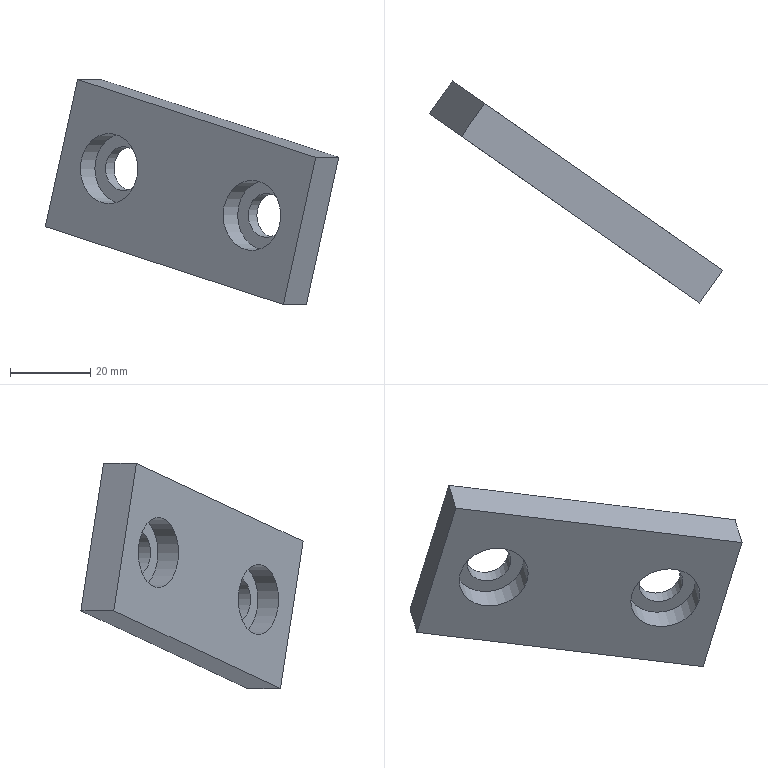Part | NX | features solid 2 | 1 solid | 12 faces | box 73.135 x 55.385 x 56.117 mm | volume 24766 mm3 | plane 8 | cylinder 4 | commonest cylinder face diameters 11 x2 17.5 x2
STEP:
#1=CARTESIAN_POINT('',(-660.026,230.842,18.06));
#2=VERTEX_POINT('',#1);
#3=CARTESIAN_POINT('',(-651.969,225.201,54.765));
#4=VERTEX_POINT('',#3);
#5=CARTESIAN_POINT('',(-681.651,245.984,-80.464));
#6=DIRECTION('',(0.212,-0.1485,0.9659));
#7=VECTOR('',#6,1000.);
#8=LINE('',#5,#7);
#9=EDGE_CURVE('',#2,#4,#8,.T.);
#10=ORIENTED_EDGE('',*,*,#9,.T.);
#11=CARTESIAN_POINT('',(-657.705,217.009,54.765));
#12=VERTEX_POINT('',#11);
#13=CARTESIAN_POINT('',(-396.728,589.724,54.765));
#14=DIRECTION('',(0.5736,0.8192,0.));
#15=VECTOR('',#14,1000.);
#16=LINE('',#13,#15);
#17=EDGE_CURVE('',#12,#4,#16,.T.);
#18=ORIENTED_EDGE('',*,*,#17,.F.);
#19=CARTESIAN_POINT('',(-665.761,222.651,18.06));
#20=VERTEX_POINT('',#19);
#21=CARTESIAN_POINT('',(-687.387,237.793,-80.464));
#22=DIRECTION('',(0.212,-0.1485,0.9659));
#23=VECTOR('',#22,1000.);
#24=LINE('',#21,#23);
#25=EDGE_CURVE('',#20,#12,#24,.T.);
#26=ORIENTED_EDGE('',*,*,#25,.F.);
#27=CARTESIAN_POINT('',(-404.784,595.365,18.06));
#28=DIRECTION('',(0.5736,0.8192,0.));
#29=VECTOR('',#28,1000.);
#30=LINE('',#27,#29);
#31=EDGE_CURVE('',#20,#2,#30,.T.);
#32=ORIENTED_EDGE('',*,*,#31,.T.);
#33=EDGE_LOOP('',(#10,#18,#26,#32));
#34=FACE_BOUND('',#33,.T.);
#35=CARTESIAN_POINT('',(-690.254,233.697,-80.464));
#36=DIRECTION('',(0.7912,-0.554,-0.2588));
#37=DIRECTION('',(-0.5736,-0.8192,0.));
#38=AXIS2_PLACEMENT_3D('',#35,#36,#37);
#39=PLANE('',#38);
#40=ADVANCED_FACE('',(#34),#39,.T.);
#41=CARTESIAN_POINT('',(-719.369,272.394,37.472));
#42=VERTEX_POINT('',#41);
#43=CARTESIAN_POINT('',(-760.909,301.481,51.06));
#44=DIRECTION('',(0.7912,-0.554,-0.2588));
#45=VECTOR('',#44,1000.);
#46=LINE('',#43,#45);
#47=EDGE_CURVE('',#42,#2,#46,.T.);
#48=ORIENTED_EDGE('',*,*,#47,.T.);
#49=ORIENTED_EDGE('',*,*,#31,.F.);
#50=CARTESIAN_POINT('',(-725.104,264.203,37.472));
#51=VERTEX_POINT('',#50);
#52=CARTESIAN_POINT('',(-766.644,293.29,51.06));
#53=DIRECTION('',(0.7912,-0.554,-0.2588));
#54=VECTOR('',#53,1000.);
#55=LINE('',#52,#54);
#56=EDGE_CURVE('',#51,#20,#55,.T.);
#57=ORIENTED_EDGE('',*,*,#56,.F.);
#58=CARTESIAN_POINT('',(-727.972,260.107,37.472));
#59=DIRECTION('',(0.5736,0.8192,0.));
#60=VECTOR('',#59,1000.);
#61=LINE('',#58,#60);
#62=EDGE_CURVE('',#51,#42,#61,.T.);
#63=ORIENTED_EDGE('',*,*,#62,.T.);
#64=EDGE_LOOP('',(#48,#49,#57,#63));
#65=FACE_BOUND('',#64,.T.);
#66=CARTESIAN_POINT('',(-505.667,666.004,51.06));
#67=DIRECTION('',(-0.212,0.1485,-0.9659));
#68=DIRECTION('',(-0.1706,0.9676,0.1862));
#69=AXIS2_PLACEMENT_3D('',#66,#67,#68);
#70=PLANE('',#69);
#71=ADVANCED_FACE('',(#65),#70,.T.);
#72=CARTESIAN_POINT('',(-711.312,266.753,74.177));
#73=VERTEX_POINT('',#72);
#74=CARTESIAN_POINT('',(-731.61,280.966,-18.302));
#75=DIRECTION('',(0.212,-0.1485,0.9659));
#76=VECTOR('',#75,1000.);
#77=LINE('',#74,#76);
#78=EDGE_CURVE('',#42,#73,#77,.T.);
#79=ORIENTED_EDGE('',*,*,#78,.F.);
#80=ORIENTED_EDGE('',*,*,#62,.F.);
#81=CARTESIAN_POINT('',(-717.048,258.562,74.177));
#82=VERTEX_POINT('',#81);
#83=CARTESIAN_POINT('',(-737.346,272.775,-18.302));
#84=DIRECTION('',(0.212,-0.1485,0.9659));
#85=VECTOR('',#84,1000.);
#86=LINE('',#83,#85);
#87=EDGE_CURVE('',#51,#82,#86,.T.);
#88=ORIENTED_EDGE('',*,*,#87,.T.);
#89=CARTESIAN_POINT('',(-719.916,254.466,74.177));
#90=DIRECTION('',(0.5736,0.8192,0.));
#91=VECTOR('',#90,1000.);
#92=LINE('',#89,#91);
#93=EDGE_CURVE('',#82,#73,#92,.T.);
#94=ORIENTED_EDGE('',*,*,#93,.T.);
#95=EDGE_LOOP('',(#79,#80,#88,#94));
#96=FACE_BOUND('',#95,.T.);
#97=CARTESIAN_POINT('',(-749.597,275.249,-61.053));
#98=DIRECTION('',(0.7912,-0.554,-0.2588));
#99=DIRECTION('',(-0.5736,-0.8192,0.));
#100=AXIS2_PLACEMENT_3D('',#97,#98,#99);
#101=PLANE('',#100);
#102=ADVANCED_FACE('',(#96),#101,.F.);
#103=CARTESIAN_POINT('',(-752.852,295.84,87.765));
#104=DIRECTION('',(0.7912,-0.554,-0.2588));
#105=VECTOR('',#104,1000.);
#106=LINE('',#103,#105);
#107=EDGE_CURVE('',#73,#4,#106,.T.);
#108=ORIENTED_EDGE('',*,*,#107,.F.);
#109=ORIENTED_EDGE('',*,*,#93,.F.);
#110=CARTESIAN_POINT('',(-758.588,287.648,87.765));
#111=DIRECTION('',(0.7912,-0.554,-0.2588));
#112=VECTOR('',#111,1000.);
#113=LINE('',#110,#112);
#114=EDGE_CURVE('',#82,#12,#113,.T.);
#115=ORIENTED_EDGE('',*,*,#114,.T.);
#116=ORIENTED_EDGE('',*,*,#17,.T.);
#117=EDGE_LOOP('',(#108,#109,#115,#116));
#118=FACE_BOUND('',#117,.T.);
#119=CARTESIAN_POINT('',(-497.611,660.363,87.765));
#120=DIRECTION('',(-0.212,0.1485,-0.9659));
#121=DIRECTION('',(-0.1706,0.9676,0.1862));
#122=AXIS2_PLACEMENT_3D('',#119,#120,#121);
#123=PLANE('',#122);
#124=ADVANCED_FACE('',(#118),#123,.F.);
#125=CARTESIAN_POINT('',(-680.769,233.159,40.295));
#126=VERTEX_POINT('',#125);
#127=CARTESIAN_POINT('',(-673.602,228.14,40.295));
#128=DIRECTION('',(0.5736,0.8192,0.));
#129=DIRECTION('',(-0.8192,0.5736,0.));
#130=AXIS2_PLACEMENT_3D('',#127,#128,#129);
#131=CIRCLE('',#130,8.75);
#132=EDGE_CURVE('',#126,#126,#131,.T.);
#133=ORIENTED_EDGE('',*,*,#132,.T.);
#134=EDGE_LOOP('',(#133));
#135=FACE_BOUND('',#134,.T.);
#136=CARTESIAN_POINT('',(-716.375,258.091,51.942));
#137=VERTEX_POINT('',#136);
#138=CARTESIAN_POINT('',(-709.207,253.072,51.942));
#139=DIRECTION('',(0.5736,0.8192,0.));
#140=DIRECTION('',(-0.8192,0.5736,0.));
#141=AXIS2_PLACEMENT_3D('',#138,#139,#140);
#142=CIRCLE('',#141,8.75);
#143=EDGE_CURVE('',#137,#137,#142,.T.);
#144=ORIENTED_EDGE('',*,*,#143,.T.);
#145=EDGE_LOOP('',(#144));
#146=FACE_BOUND('',#145,.T.);
#147=ORIENTED_EDGE('',*,*,#25,.T.);
#148=ORIENTED_EDGE('',*,*,#114,.F.);
#149=ORIENTED_EDGE('',*,*,#87,.F.);
#150=ORIENTED_EDGE('',*,*,#56,.T.);
#151=EDGE_LOOP('',(#147,#148,#149,#150));
#152=FACE_BOUND('',#151,.T.);
#153=CARTESIAN_POINT('',(-739.324,274.16,-17.655));
#154=DIRECTION('',(-0.5736,-0.8192,0.));
#155=DIRECTION('',(-0.8192,0.5736,0.));
#156=AXIS2_PLACEMENT_3D('',#153,#154,#155);
#157=PLANE('',#156);
#158=ADVANCED_FACE('',(#135,#146,#152),#157,.T.);
#159=CARTESIAN_POINT('',(-663.361,233.177,40.295));
#160=VERTEX_POINT('',#159);
#161=CARTESIAN_POINT('',(-667.866,236.332,40.295));
#162=DIRECTION('',(-0.5736,-0.8192,0.));
#163=DIRECTION('',(0.8192,-0.5736,0.));
#164=AXIS2_PLACEMENT_3D('',#161,#162,#163);
#165=CIRCLE('',#164,5.5);
#166=EDGE_CURVE('',#160,#160,#165,.T.);
#167=ORIENTED_EDGE('',*,*,#166,.T.);
#168=EDGE_LOOP('',(#167));
#169=FACE_BOUND('',#168,.T.);
#170=CARTESIAN_POINT('',(-698.966,258.109,51.942));
#171=VERTEX_POINT('',#170);
#172=CARTESIAN_POINT('',(-703.472,261.263,51.942));
#173=DIRECTION('',(-0.5736,-0.8192,0.));
#174=DIRECTION('',(0.8192,-0.5736,0.));
#175=AXIS2_PLACEMENT_3D('',#172,#173,#174);
#176=CIRCLE('',#175,5.5);
#177=EDGE_CURVE('',#171,#171,#176,.T.);
#178=ORIENTED_EDGE('',*,*,#177,.T.);
#179=EDGE_LOOP('',(#178));
#180=FACE_BOUND('',#179,.T.);
#181=ORIENTED_EDGE('',*,*,#9,.F.);
#182=ORIENTED_EDGE('',*,*,#47,.F.);
#183=ORIENTED_EDGE('',*,*,#78,.T.);
#184=ORIENTED_EDGE('',*,*,#107,.T.);
#185=EDGE_LOOP('',(#181,#182,#183,#184));
#186=FACE_BOUND('',#185,.T.);
#187=CARTESIAN_POINT('',(-733.588,282.351,-17.655));
#188=DIRECTION('',(-0.5736,-0.8192,0.));
#189=DIRECTION('',(-0.8192,0.5736,0.));
#190=AXIS2_PLACEMENT_3D('',#187,#188,#189);
#191=PLANE('',#190);
#192=ADVANCED_FACE('',(#169,#180,#186),#191,.F.);
#193=CARTESIAN_POINT('',(-710.099,261.387,51.942));
#194=VERTEX_POINT('',#193);
#195=CARTESIAN_POINT('',(-705.594,258.233,51.942));
#196=DIRECTION('',(0.5736,0.8192,0.));
#197=DIRECTION('',(-0.8192,0.5736,0.));
#198=AXIS2_PLACEMENT_3D('',#195,#196,#197);
#199=CIRCLE('',#198,5.5);
#200=EDGE_CURVE('',#194,#194,#199,.T.);
#201=ORIENTED_EDGE('',*,*,#200,.F.);
#202=EDGE_LOOP('',(#201));
#203=FACE_BOUND('',#202,.T.);
#204=ORIENTED_EDGE('',*,*,#177,.F.);
#205=EDGE_LOOP('',(#204));
#206=FACE_BOUND('',#205,.T.);
#207=CARTESIAN_POINT('',(-680.529,294.029,51.942));
#208=DIRECTION('',(0.5736,0.8192,0.));
#209=DIRECTION('',(-0.8192,0.5736,0.));
#210=AXIS2_PLACEMENT_3D('',#207,#208,#209);
#211=CYLINDRICAL_SURFACE('',#210,5.5);
#212=ADVANCED_FACE('',(#203,#206),#211,.F.);
#213=ORIENTED_EDGE('',*,*,#200,.T.);
#214=EDGE_LOOP('',(#213));
#215=FACE_BOUND('',#214,.T.);
#216=CARTESIAN_POINT('',(-712.762,263.251,51.942));
#217=VERTEX_POINT('',#216);
#218=CARTESIAN_POINT('',(-705.594,258.233,51.942));
#219=DIRECTION('',(0.5736,0.8192,0.));
#220=DIRECTION('',(-0.8192,0.5736,0.));
#221=AXIS2_PLACEMENT_3D('',#218,#219,#220);
#222=CIRCLE('',#221,8.75);
#223=EDGE_CURVE('',#217,#217,#222,.T.);
#224=ORIENTED_EDGE('',*,*,#223,.F.);
#225=EDGE_LOOP('',(#224));
#226=FACE_BOUND('',#225,.T.);
#227=CARTESIAN_POINT('',(-697.682,252.692,49.354));
#228=DIRECTION('',(0.5736,0.8192,0.));
#229=DIRECTION('',(-0.8192,0.5736,0.));
#230=AXIS2_PLACEMENT_3D('',#227,#228,#229);
#231=PLANE('',#230);
#232=ADVANCED_FACE('',(#215,#226),#231,.F.);
#233=ORIENTED_EDGE('',*,*,#223,.T.);
#234=EDGE_LOOP('',(#233));
#235=FACE_BOUND('',#234,.T.);
#236=ORIENTED_EDGE('',*,*,#143,.F.);
#237=EDGE_LOOP('',(#236));
#238=FACE_BOUND('',#237,.T.);
#239=CARTESIAN_POINT('',(-709.207,253.072,51.942));
#240=DIRECTION('',(0.5736,0.8192,0.));
#241=DIRECTION('',(-0.8192,0.5736,0.));
#242=AXIS2_PLACEMENT_3D('',#239,#240,#241);
#243=CYLINDRICAL_SURFACE('',#242,8.75);
#244=ADVANCED_FACE('',(#235,#238),#243,.F.);
#245=CARTESIAN_POINT('',(-674.493,236.456,40.295));
#246=VERTEX_POINT('',#245);
#247=CARTESIAN_POINT('',(-669.988,233.301,40.295));
#248=DIRECTION('',(0.5736,0.8192,0.));
#249=DIRECTION('',(-0.8192,0.5736,0.));
#250=AXIS2_PLACEMENT_3D('',#247,#248,#249);
#251=CIRCLE('',#250,5.5);
#252=EDGE_CURVE('',#246,#246,#251,.T.);
#253=ORIENTED_EDGE('',*,*,#252,.F.);
#254=EDGE_LOOP('',(#253));
#255=FACE_BOUND('',#254,.T.);
#256=ORIENTED_EDGE('',*,*,#166,.F.);
#257=EDGE_LOOP('',(#256));
#258=FACE_BOUND('',#257,.T.);
#259=CARTESIAN_POINT('',(-644.923,269.098,40.295));
#260=DIRECTION('',(0.5736,0.8192,0.));
#261=DIRECTION('',(-0.8192,0.5736,0.));
#262=AXIS2_PLACEMENT_3D('',#259,#260,#261);
#263=CYLINDRICAL_SURFACE('',#262,5.5);
#264=ADVANCED_FACE('',(#255,#258),#263,.F.);
#265=ORIENTED_EDGE('',*,*,#252,.T.);
#266=EDGE_LOOP('',(#265));
#267=FACE_BOUND('',#266,.T.);
#268=CARTESIAN_POINT('',(-677.156,238.32,40.295));
#269=VERTEX_POINT('',#268);
#270=CARTESIAN_POINT('',(-669.988,233.301,40.295));
#271=DIRECTION('',(0.5736,0.8192,0.));
#272=DIRECTION('',(-0.8192,0.5736,0.));
#273=AXIS2_PLACEMENT_3D('',#270,#271,#272);
#274=CIRCLE('',#273,8.75);
#275=EDGE_CURVE('',#269,#269,#274,.T.);
#276=ORIENTED_EDGE('',*,*,#275,.F.);
#277=EDGE_LOOP('',(#276));
#278=FACE_BOUND('',#277,.T.);
#279=CARTESIAN_POINT('',(-677.901,238.841,42.883));
#280=DIRECTION('',(0.5736,0.8192,0.));
#281=DIRECTION('',(-0.8192,0.5736,0.));
#282=AXIS2_PLACEMENT_3D('',#279,#280,#281);
#283=PLANE('',#282);
#284=ADVANCED_FACE('',(#267,#278),#283,.F.);
#285=ORIENTED_EDGE('',*,*,#275,.T.);
#286=EDGE_LOOP('',(#285));
#287=FACE_BOUND('',#286,.T.);
#288=ORIENTED_EDGE('',*,*,#132,.F.);
#289=EDGE_LOOP('',(#288));
#290=FACE_BOUND('',#289,.T.);
#291=CARTESIAN_POINT('',(-673.602,228.14,40.295));
#292=DIRECTION('',(0.5736,0.8192,0.));
#293=DIRECTION('',(-0.8192,0.5736,0.));
#294=AXIS2_PLACEMENT_3D('',#291,#292,#293);
#295=CYLINDRICAL_SURFACE('',#294,8.75);
#296=ADVANCED_FACE('',(#287,#290),#295,.F.);
#297=CLOSED_SHELL('',(#40,#71,#102,#124,#158,#192,#212,#232,#244,#264,#284,#296));
#298=MANIFOLD_SOLID_BREP('',#297);
#299=(LENGTH_UNIT()NAMED_UNIT(*)SI_UNIT(.MILLI.,.METRE.));
#300=UNCERTAINTY_MEASURE_WITH_UNIT(LENGTH_MEASURE(0.00001),#299,'','');
#301=(NAMED_UNIT(*)PLANE_ANGLE_UNIT()SI_UNIT($,.RADIAN.));
#302=(NAMED_UNIT(*)SI_UNIT($,.STERADIAN.)SOLID_ANGLE_UNIT());
#303=(GEOMETRIC_REPRESENTATION_CONTEXT(3)GLOBAL_UNCERTAINTY_ASSIGNED_CONTEXT((#300))GLOBAL_UNIT_ASSIGNED_CONTEXT((#299,#301,#302))REPRESENTATION_CONTEXT('',''));
#304=ADVANCED_BREP_SHAPE_REPRESENTATION('',(#298),#303);